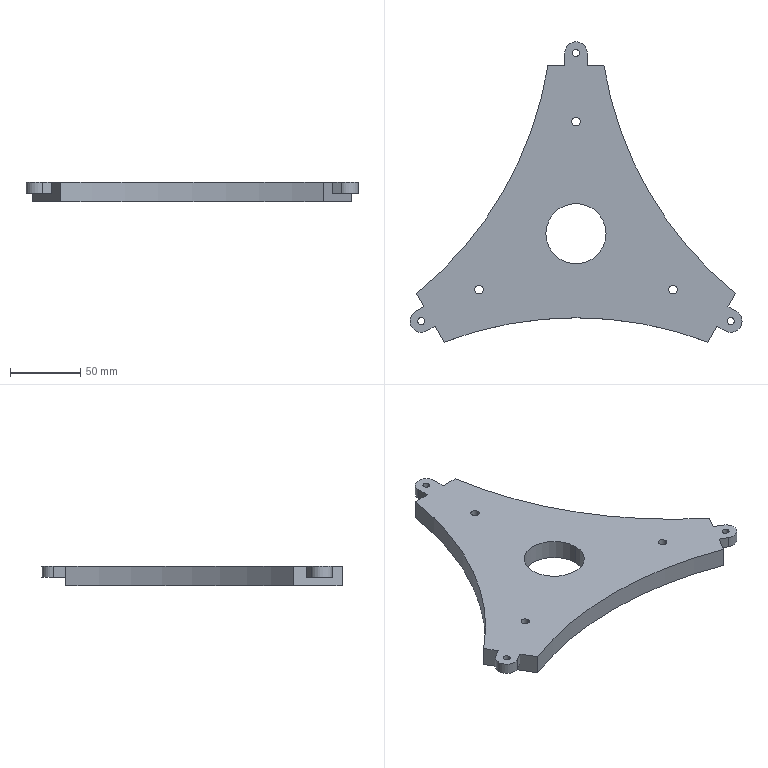Part | SolidWorks | features ICE 3, 3DProfileFeature 2, HoleWzd 2, CirPattern 1, Extrusion 1 | 1 solid | 35 faces | box 237.049 x 214.321 x 14 mm | volume 297445 mm3 | cylinder 21 | plane 14 | commonest cylinder face diameters 5 x6 6 x6 16 x4 526.632 x3 43 x2
STEP:
#1=CARTESIAN_POINT('',(-3.,80.,14.));
#2=VERTEX_POINT('',#1);
#3=CARTESIAN_POINT('',(3.,80.,14.));
#4=VERTEX_POINT('',#3);
#5=CARTESIAN_POINT('',(0.,80.,14.));
#6=DIRECTION('',(0.,0.,1.));
#7=DIRECTION('',(1.,0.,0.));
#8=AXIS2_PLACEMENT_3D('',#5,#6,#7);
#9=CIRCLE('',#8,3.);
#10=EDGE_CURVE('',#2,#4,#9,.T.);
#11=ORIENTED_EDGE('',*,*,#10,.T.);
#12=CARTESIAN_POINT('',(3.,80.,0.));
#13=VERTEX_POINT('',#12);
#14=CARTESIAN_POINT('',(3.,80.,17.));
#15=DIRECTION('',(0.,0.,-1.));
#16=VECTOR('',#15,1000.);
#17=LINE('',#14,#16);
#18=EDGE_CURVE('',#4,#13,#17,.T.);
#19=ORIENTED_EDGE('',*,*,#18,.T.);
#20=CARTESIAN_POINT('',(-3.,80.,0.));
#21=VERTEX_POINT('',#20);
#22=CARTESIAN_POINT('',(0.,80.,0.));
#23=DIRECTION('',(0.,0.,-1.));
#24=DIRECTION('',(-1.,0.,0.));
#25=AXIS2_PLACEMENT_3D('',#22,#23,#24);
#26=CIRCLE('',#25,3.);
#27=EDGE_CURVE('',#13,#21,#26,.T.);
#28=ORIENTED_EDGE('',*,*,#27,.T.);
#29=CARTESIAN_POINT('',(-3.,80.,17.));
#30=DIRECTION('',(0.,0.,-1.));
#31=VECTOR('',#30,1000.);
#32=LINE('',#29,#31);
#33=EDGE_CURVE('',#2,#21,#32,.T.);
#34=ORIENTED_EDGE('',*,*,#33,.F.);
#35=EDGE_LOOP('',(#11,#19,#28,#34));
#36=FACE_OUTER_BOUND('',#35,.T.);
#37=CARTESIAN_POINT('',(0.,80.,17.));
#38=DIRECTION('',(0.,0.,-1.));
#39=DIRECTION('',(-1.,0.,0.));
#40=AXIS2_PLACEMENT_3D('',#37,#38,#39);
#41=CYLINDRICAL_SURFACE('',#40,3.);
#42=ADVANCED_FACE('',(#36),#41,.F.);
#43=CARTESIAN_POINT('',(-72.282,-40.,14.));
#44=VERTEX_POINT('',#43);
#45=CARTESIAN_POINT('',(-66.282,-40.,14.));
#46=VERTEX_POINT('',#45);
#47=CARTESIAN_POINT('',(-69.282,-40.,14.));
#48=DIRECTION('',(0.,0.,1.));
#49=DIRECTION('',(1.,0.,0.));
#50=AXIS2_PLACEMENT_3D('',#47,#48,#49);
#51=CIRCLE('',#50,3.);
#52=EDGE_CURVE('',#44,#46,#51,.T.);
#53=ORIENTED_EDGE('',*,*,#52,.T.);
#54=CARTESIAN_POINT('',(-66.282,-40.,0.));
#55=VERTEX_POINT('',#54);
#56=CARTESIAN_POINT('',(-66.282,-40.,17.));
#57=DIRECTION('',(0.,0.,-1.));
#58=VECTOR('',#57,1000.);
#59=LINE('',#56,#58);
#60=EDGE_CURVE('',#46,#55,#59,.T.);
#61=ORIENTED_EDGE('',*,*,#60,.T.);
#62=CARTESIAN_POINT('',(-72.282,-40.,0.));
#63=VERTEX_POINT('',#62);
#64=CARTESIAN_POINT('',(-69.282,-40.,0.));
#65=DIRECTION('',(0.,0.,-1.));
#66=DIRECTION('',(-1.,0.,0.));
#67=AXIS2_PLACEMENT_3D('',#64,#65,#66);
#68=CIRCLE('',#67,3.);
#69=EDGE_CURVE('',#55,#63,#68,.T.);
#70=ORIENTED_EDGE('',*,*,#69,.T.);
#71=CARTESIAN_POINT('',(-72.282,-40.,17.));
#72=DIRECTION('',(0.,0.,-1.));
#73=VECTOR('',#72,1000.);
#74=LINE('',#71,#73);
#75=EDGE_CURVE('',#44,#63,#74,.T.);
#76=ORIENTED_EDGE('',*,*,#75,.F.);
#77=EDGE_LOOP('',(#53,#61,#70,#76));
#78=FACE_OUTER_BOUND('',#77,.T.);
#79=CARTESIAN_POINT('',(-69.282,-40.,17.));
#80=DIRECTION('',(0.,0.,-1.));
#81=DIRECTION('',(-1.,0.,0.));
#82=AXIS2_PLACEMENT_3D('',#79,#80,#81);
#83=CYLINDRICAL_SURFACE('',#82,3.);
#84=ADVANCED_FACE('',(#78),#83,.F.);
#85=CARTESIAN_POINT('',(66.282,-40.,14.));
#86=VERTEX_POINT('',#85);
#87=CARTESIAN_POINT('',(72.282,-40.,14.));
#88=VERTEX_POINT('',#87);
#89=CARTESIAN_POINT('',(69.282,-40.,14.));
#90=DIRECTION('',(0.,0.,1.));
#91=DIRECTION('',(1.,0.,0.));
#92=AXIS2_PLACEMENT_3D('',#89,#90,#91);
#93=CIRCLE('',#92,3.);
#94=EDGE_CURVE('',#86,#88,#93,.T.);
#95=ORIENTED_EDGE('',*,*,#94,.T.);
#96=CARTESIAN_POINT('',(72.282,-40.,0.));
#97=VERTEX_POINT('',#96);
#98=CARTESIAN_POINT('',(72.282,-40.,17.));
#99=DIRECTION('',(0.,0.,-1.));
#100=VECTOR('',#99,1000.);
#101=LINE('',#98,#100);
#102=EDGE_CURVE('',#88,#97,#101,.T.);
#103=ORIENTED_EDGE('',*,*,#102,.T.);
#104=CARTESIAN_POINT('',(66.282,-40.,0.));
#105=VERTEX_POINT('',#104);
#106=CARTESIAN_POINT('',(69.282,-40.,0.));
#107=DIRECTION('',(0.,0.,-1.));
#108=DIRECTION('',(-1.,0.,0.));
#109=AXIS2_PLACEMENT_3D('',#106,#107,#108);
#110=CIRCLE('',#109,3.);
#111=EDGE_CURVE('',#97,#105,#110,.T.);
#112=ORIENTED_EDGE('',*,*,#111,.T.);
#113=CARTESIAN_POINT('',(66.282,-40.,17.));
#114=DIRECTION('',(0.,0.,-1.));
#115=VECTOR('',#114,1000.);
#116=LINE('',#113,#115);
#117=EDGE_CURVE('',#86,#105,#116,.T.);
#118=ORIENTED_EDGE('',*,*,#117,.F.);
#119=EDGE_LOOP('',(#95,#103,#112,#118));
#120=FACE_OUTER_BOUND('',#119,.T.);
#121=CARTESIAN_POINT('',(69.282,-40.,17.));
#122=DIRECTION('',(0.,0.,-1.));
#123=DIRECTION('',(-1.,0.,0.));
#124=AXIS2_PLACEMENT_3D('',#121,#122,#123);
#125=CYLINDRICAL_SURFACE('',#124,3.);
#126=ADVANCED_FACE('',(#120),#125,.F.);
#127=CARTESIAN_POINT('',(-113.024,-62.434,6.));
#128=VERTEX_POINT('',#127);
#129=CARTESIAN_POINT('',(-108.024,-62.434,6.));
#130=VERTEX_POINT('',#129);
#131=CARTESIAN_POINT('',(-110.524,-62.434,6.));
#132=DIRECTION('',(0.,0.,1.));
#133=DIRECTION('',(1.,0.,0.));
#134=AXIS2_PLACEMENT_3D('',#131,#132,#133);
#135=CIRCLE('',#134,2.5);
#136=EDGE_CURVE('',#128,#130,#135,.T.);
#137=ORIENTED_EDGE('',*,*,#136,.F.);
#138=CARTESIAN_POINT('',(-113.024,-62.434,14.));
#139=VERTEX_POINT('',#138);
#140=CARTESIAN_POINT('',(-113.024,-62.434,14.));
#141=DIRECTION('',(0.,0.,1.));
#142=VECTOR('',#141,1000.);
#143=LINE('',#140,#142);
#144=EDGE_CURVE('',#128,#139,#143,.T.);
#145=ORIENTED_EDGE('',*,*,#144,.T.);
#146=CARTESIAN_POINT('',(-108.024,-62.434,14.));
#147=VERTEX_POINT('',#146);
#148=CARTESIAN_POINT('',(-110.524,-62.434,14.));
#149=DIRECTION('',(0.,0.,1.));
#150=DIRECTION('',(1.,0.,0.));
#151=AXIS2_PLACEMENT_3D('',#148,#149,#150);
#152=CIRCLE('',#151,2.5);
#153=EDGE_CURVE('',#139,#147,#152,.T.);
#154=ORIENTED_EDGE('',*,*,#153,.T.);
#155=CARTESIAN_POINT('',(-108.024,-62.434,14.));
#156=DIRECTION('',(0.,0.,1.));
#157=VECTOR('',#156,1000.);
#158=LINE('',#155,#157);
#159=EDGE_CURVE('',#130,#147,#158,.T.);
#160=ORIENTED_EDGE('',*,*,#159,.F.);
#161=EDGE_LOOP('',(#137,#145,#154,#160));
#162=FACE_OUTER_BOUND('',#161,.T.);
#163=CARTESIAN_POINT('',(-110.524,-62.434,14.));
#164=DIRECTION('',(0.,0.,1.));
#165=DIRECTION('',(1.,0.,0.));
#166=AXIS2_PLACEMENT_3D('',#163,#164,#165);
#167=CYLINDRICAL_SURFACE('',#166,2.5);
#168=ADVANCED_FACE('',(#162),#167,.F.);
#169=CARTESIAN_POINT('',(108.024,-62.434,6.));
#170=VERTEX_POINT('',#169);
#171=CARTESIAN_POINT('',(113.024,-62.434,6.));
#172=VERTEX_POINT('',#171);
#173=CARTESIAN_POINT('',(110.524,-62.434,6.));
#174=DIRECTION('',(0.,0.,1.));
#175=DIRECTION('',(1.,0.,0.));
#176=AXIS2_PLACEMENT_3D('',#173,#174,#175);
#177=CIRCLE('',#176,2.5);
#178=EDGE_CURVE('',#170,#172,#177,.T.);
#179=ORIENTED_EDGE('',*,*,#178,.F.);
#180=CARTESIAN_POINT('',(108.024,-62.434,14.));
#181=VERTEX_POINT('',#180);
#182=CARTESIAN_POINT('',(108.024,-62.434,14.));
#183=DIRECTION('',(0.,0.,1.));
#184=VECTOR('',#183,1000.);
#185=LINE('',#182,#184);
#186=EDGE_CURVE('',#170,#181,#185,.T.);
#187=ORIENTED_EDGE('',*,*,#186,.T.);
#188=CARTESIAN_POINT('',(113.024,-62.434,14.));
#189=VERTEX_POINT('',#188);
#190=CARTESIAN_POINT('',(110.524,-62.434,14.));
#191=DIRECTION('',(0.,0.,1.));
#192=DIRECTION('',(1.,0.,0.));
#193=AXIS2_PLACEMENT_3D('',#190,#191,#192);
#194=CIRCLE('',#193,2.5);
#195=EDGE_CURVE('',#181,#189,#194,.T.);
#196=ORIENTED_EDGE('',*,*,#195,.T.);
#197=CARTESIAN_POINT('',(113.024,-62.434,14.));
#198=DIRECTION('',(0.,0.,1.));
#199=VECTOR('',#198,1000.);
#200=LINE('',#197,#199);
#201=EDGE_CURVE('',#172,#189,#200,.T.);
#202=ORIENTED_EDGE('',*,*,#201,.F.);
#203=EDGE_LOOP('',(#179,#187,#196,#202));
#204=FACE_OUTER_BOUND('',#203,.T.);
#205=CARTESIAN_POINT('',(110.524,-62.434,14.));
#206=DIRECTION('',(0.,0.,1.));
#207=DIRECTION('',(1.,0.,0.));
#208=AXIS2_PLACEMENT_3D('',#205,#206,#207);
#209=CYLINDRICAL_SURFACE('',#208,2.5);
#210=ADVANCED_FACE('',(#204),#209,.F.);
#211=CARTESIAN_POINT('',(21.5,0.,14.));
#212=VERTEX_POINT('',#211);
#213=CARTESIAN_POINT('',(-21.5,0.,14.));
#214=VERTEX_POINT('',#213);
#215=CARTESIAN_POINT('',(0.,0.,14.));
#216=DIRECTION('',(0.,0.,-1.));
#217=DIRECTION('',(-1.,0.,0.));
#218=AXIS2_PLACEMENT_3D('',#215,#216,#217);
#219=CIRCLE('',#218,21.5);
#220=EDGE_CURVE('',#212,#214,#219,.T.);
#221=ORIENTED_EDGE('',*,*,#220,.F.);
#222=CARTESIAN_POINT('',(21.5,0.,0.));
#223=VERTEX_POINT('',#222);
#224=CARTESIAN_POINT('',(21.5,0.,14.));
#225=DIRECTION('',(0.,0.,-1.));
#226=VECTOR('',#225,1000.);
#227=LINE('',#224,#226);
#228=EDGE_CURVE('',#212,#223,#227,.T.);
#229=ORIENTED_EDGE('',*,*,#228,.T.);
#230=CARTESIAN_POINT('',(-21.5,0.,0.));
#231=VERTEX_POINT('',#230);
#232=CARTESIAN_POINT('',(0.,0.,0.));
#233=DIRECTION('',(0.,0.,-1.));
#234=DIRECTION('',(-1.,0.,0.));
#235=AXIS2_PLACEMENT_3D('',#232,#233,#234);
#236=CIRCLE('',#235,21.5);
#237=EDGE_CURVE('',#223,#231,#236,.T.);
#238=ORIENTED_EDGE('',*,*,#237,.T.);
#239=CARTESIAN_POINT('',(-21.5,0.,14.));
#240=DIRECTION('',(0.,0.,-1.));
#241=VECTOR('',#240,1000.);
#242=LINE('',#239,#241);
#243=EDGE_CURVE('',#214,#231,#242,.T.);
#244=ORIENTED_EDGE('',*,*,#243,.F.);
#245=EDGE_LOOP('',(#221,#229,#238,#244));
#246=FACE_OUTER_BOUND('',#245,.T.);
#247=CARTESIAN_POINT('',(0.,0.,14.));
#248=DIRECTION('',(0.,0.,-1.));
#249=DIRECTION('',(-1.,0.,0.));
#250=AXIS2_PLACEMENT_3D('',#247,#248,#249);
#251=CYLINDRICAL_SURFACE('',#250,21.5);
#252=ADVANCED_FACE('',(#246),#251,.F.);
#253=CARTESIAN_POINT('',(-2.5,129.,14.));
#254=VERTEX_POINT('',#253);
#255=CARTESIAN_POINT('',(2.5,129.,14.));
#256=VERTEX_POINT('',#255);
#257=CARTESIAN_POINT('',(0.,129.,14.));
#258=DIRECTION('',(0.,0.,1.));
#259=DIRECTION('',(1.,0.,0.));
#260=AXIS2_PLACEMENT_3D('',#257,#258,#259);
#261=CIRCLE('',#260,2.5);
#262=EDGE_CURVE('',#254,#256,#261,.T.);
#263=ORIENTED_EDGE('',*,*,#262,.T.);
#264=CARTESIAN_POINT('',(2.5,129.,6.));
#265=VERTEX_POINT('',#264);
#266=CARTESIAN_POINT('',(2.5,129.,6.));
#267=DIRECTION('',(0.,0.,-1.));
#268=VECTOR('',#267,1000.);
#269=LINE('',#266,#268);
#270=EDGE_CURVE('',#256,#265,#269,.T.);
#271=ORIENTED_EDGE('',*,*,#270,.T.);
#272=CARTESIAN_POINT('',(-2.5,129.,6.));
#273=VERTEX_POINT('',#272);
#274=CARTESIAN_POINT('',(0.,129.,6.));
#275=DIRECTION('',(0.,0.,-1.));
#276=DIRECTION('',(-1.,0.,0.));
#277=AXIS2_PLACEMENT_3D('',#274,#275,#276);
#278=CIRCLE('',#277,2.5);
#279=EDGE_CURVE('',#265,#273,#278,.T.);
#280=ORIENTED_EDGE('',*,*,#279,.T.);
#281=CARTESIAN_POINT('',(-2.5,129.,6.));
#282=DIRECTION('',(0.,0.,-1.));
#283=VECTOR('',#282,1000.);
#284=LINE('',#281,#283);
#285=EDGE_CURVE('',#254,#273,#284,.T.);
#286=ORIENTED_EDGE('',*,*,#285,.F.);
#287=EDGE_LOOP('',(#263,#271,#280,#286));
#288=FACE_OUTER_BOUND('',#287,.T.);
#289=CARTESIAN_POINT('',(0.,129.,6.));
#290=DIRECTION('',(0.,0.,-1.));
#291=DIRECTION('',(-1.,0.,0.));
#292=AXIS2_PLACEMENT_3D('',#289,#290,#291);
#293=CYLINDRICAL_SURFACE('',#292,2.5);
#294=ADVANCED_FACE('',(#288),#293,.F.);
#295=CARTESIAN_POINT('',(106.524,-69.362,6.));
#296=VERTEX_POINT('',#295);
#297=CARTESIAN_POINT('',(118.524,-62.434,6.));
#298=VERTEX_POINT('',#297);
#299=CARTESIAN_POINT('',(110.524,-62.434,6.));
#300=DIRECTION('',(0.,0.,1.));
#301=DIRECTION('',(-0.5,-0.866,0.));
#302=AXIS2_PLACEMENT_3D('',#299,#300,#301);
#303=CIRCLE('',#302,8.);
#304=EDGE_CURVE('',#296,#298,#303,.T.);
#305=ORIENTED_EDGE('',*,*,#304,.T.);
#306=CARTESIAN_POINT('',(118.524,-62.434,14.));
#307=VERTEX_POINT('',#306);
#308=CARTESIAN_POINT('',(118.524,-62.434,6.));
#309=DIRECTION('',(0.,0.,1.));
#310=VECTOR('',#309,1000.);
#311=LINE('',#308,#310);
#312=EDGE_CURVE('',#298,#307,#311,.T.);
#313=ORIENTED_EDGE('',*,*,#312,.T.);
#314=CARTESIAN_POINT('',(106.524,-69.362,14.));
#315=VERTEX_POINT('',#314);
#316=CARTESIAN_POINT('',(110.524,-62.434,14.));
#317=DIRECTION('',(0.,0.,1.));
#318=DIRECTION('',(-0.5,-0.866,0.));
#319=AXIS2_PLACEMENT_3D('',#316,#317,#318);
#320=CIRCLE('',#319,8.);
#321=EDGE_CURVE('',#315,#307,#320,.T.);
#322=ORIENTED_EDGE('',*,*,#321,.F.);
#323=CARTESIAN_POINT('',(106.524,-69.362,6.));
#324=DIRECTION('',(0.,0.,1.));
#325=VECTOR('',#324,1000.);
#326=LINE('',#323,#325);
#327=EDGE_CURVE('',#296,#315,#326,.T.);
#328=ORIENTED_EDGE('',*,*,#327,.F.);
#329=EDGE_LOOP('',(#305,#313,#322,#328));
#330=FACE_OUTER_BOUND('',#329,.T.);
#331=CARTESIAN_POINT('',(110.524,-62.434,6.));
#332=DIRECTION('',(0.,0.,1.));
#333=DIRECTION('',(1.,0.,0.));
#334=AXIS2_PLACEMENT_3D('',#331,#332,#333);
#335=CYLINDRICAL_SURFACE('',#334,8.);
#336=ADVANCED_FACE('',(#330),#335,.T.);
#337=CARTESIAN_POINT('',(-8.,120.,6.));
#338=VERTEX_POINT('',#337);
#339=CARTESIAN_POINT('',(-8.,120.,14.));
#340=VERTEX_POINT('',#339);
#341=CARTESIAN_POINT('',(-8.,120.,6.));
#342=DIRECTION('',(0.,0.,1.));
#343=VECTOR('',#342,1000.);
#344=LINE('',#341,#343);
#345=EDGE_CURVE('',#338,#340,#344,.T.);
#346=ORIENTED_EDGE('',*,*,#345,.F.);
#347=CARTESIAN_POINT('',(8.,120.,6.));
#348=VERTEX_POINT('',#347);
#349=CARTESIAN_POINT('',(0.,120.,6.));
#350=DIRECTION('',(-1.,0.,0.));
#351=VECTOR('',#350,1000.);
#352=LINE('',#349,#351);
#353=EDGE_CURVE('',#348,#338,#352,.T.);
#354=ORIENTED_EDGE('',*,*,#353,.F.);
#355=CARTESIAN_POINT('',(8.,120.,14.));
#356=VERTEX_POINT('',#355);
#357=CARTESIAN_POINT('',(8.,120.,6.));
#358=DIRECTION('',(0.,0.,1.));
#359=VECTOR('',#358,1000.);
#360=LINE('',#357,#359);
#361=EDGE_CURVE('',#348,#356,#360,.T.);
#362=ORIENTED_EDGE('',*,*,#361,.T.);
#363=CARTESIAN_POINT('',(20.,120.,14.));
#364=VERTEX_POINT('',#363);
#365=CARTESIAN_POINT('',(-20.,120.,14.));
#366=DIRECTION('',(-1.,0.,0.));
#367=VECTOR('',#366,1000.);
#368=LINE('',#365,#367);
#369=EDGE_CURVE('',#364,#356,#368,.T.);
#370=ORIENTED_EDGE('',*,*,#369,.F.);
#371=CARTESIAN_POINT('',(20.,120.,0.));
#372=VERTEX_POINT('',#371);
#373=CARTESIAN_POINT('',(20.,120.,14.));
#374=DIRECTION('',(0.,0.,-1.));
#375=VECTOR('',#374,1000.);
#376=LINE('',#373,#375);
#377=EDGE_CURVE('',#364,#372,#376,.T.);
#378=ORIENTED_EDGE('',*,*,#377,.T.);
#379=CARTESIAN_POINT('',(-20.,120.,0.));
#380=VERTEX_POINT('',#379);
#381=CARTESIAN_POINT('',(-20.,120.,0.));
#382=DIRECTION('',(-1.,0.,0.));
#383=VECTOR('',#382,1000.);
#384=LINE('',#381,#383);
#385=EDGE_CURVE('',#372,#380,#384,.T.);
#386=ORIENTED_EDGE('',*,*,#385,.T.);
#387=CARTESIAN_POINT('',(-20.,120.,14.));
#388=VERTEX_POINT('',#387);
#389=CARTESIAN_POINT('',(-20.,120.,14.));
#390=DIRECTION('',(0.,0.,-1.));
#391=VECTOR('',#390,1000.);
#392=LINE('',#389,#391);
#393=EDGE_CURVE('',#388,#380,#392,.T.);
#394=ORIENTED_EDGE('',*,*,#393,.F.);
#395=CARTESIAN_POINT('',(-20.,120.,14.));
#396=DIRECTION('',(-1.,0.,0.));
#397=VECTOR('',#396,1000.);
#398=LINE('',#395,#397);
#399=EDGE_CURVE('',#340,#388,#398,.T.);
#400=ORIENTED_EDGE('',*,*,#399,.F.);
#401=EDGE_LOOP('',(#346,#354,#362,#370,#378,#386,#394,#400));
#402=FACE_OUTER_BOUND('',#401,.T.);
#403=CARTESIAN_POINT('',(-20.,120.,14.));
#404=DIRECTION('',(0.,-1.,0.));
#405=DIRECTION('',(0.,0.,-1.));
#406=AXIS2_PLACEMENT_3D('',#403,#404,#405);
#407=PLANE('',#406);
#408=ADVANCED_FACE('',(#402),#407,.F.);
#409=CARTESIAN_POINT('',(113.923,-42.679,0.));
#410=VERTEX_POINT('',#409);
#411=CARTESIAN_POINT('',(280.,161.658,0.));
#412=DIRECTION('',(0.,0.,-1.));
#413=DIRECTION('',(1.,0.,0.));
#414=AXIS2_PLACEMENT_3D('',#411,#412,#413);
#415=CIRCLE('',#414,263.316);
#416=EDGE_CURVE('',#410,#372,#415,.T.);
#417=ORIENTED_EDGE('',*,*,#416,.T.);
#418=ORIENTED_EDGE('',*,*,#377,.F.);
#419=CARTESIAN_POINT('',(113.923,-42.679,14.));
#420=VERTEX_POINT('',#419);
#421=CARTESIAN_POINT('',(280.,161.658,14.));
#422=DIRECTION('',(0.,0.,-1.));
#423=DIRECTION('',(1.,0.,0.));
#424=AXIS2_PLACEMENT_3D('',#421,#422,#423);
#425=CIRCLE('',#424,263.316);
#426=EDGE_CURVE('',#420,#364,#425,.T.);
#427=ORIENTED_EDGE('',*,*,#426,.F.);
#428=CARTESIAN_POINT('',(113.923,-42.679,14.));
#429=DIRECTION('',(0.,0.,-1.));
#430=VECTOR('',#429,1000.);
#431=LINE('',#428,#430);
#432=EDGE_CURVE('',#420,#410,#431,.T.);
#433=ORIENTED_EDGE('',*,*,#432,.T.);
#434=EDGE_LOOP('',(#417,#418,#427,#433));
#435=FACE_OUTER_BOUND('',#434,.T.);
#436=CARTESIAN_POINT('',(280.,161.658,14.));
#437=DIRECTION('',(0.,0.,-1.));
#438=DIRECTION('',(-1.,0.,0.));
#439=AXIS2_PLACEMENT_3D('',#436,#437,#438);
#440=CYLINDRICAL_SURFACE('',#439,263.316);
#441=ADVANCED_FACE('',(#435),#440,.F.);
#442=CARTESIAN_POINT('',(-113.923,-42.679,0.));
#443=VERTEX_POINT('',#442);
#444=CARTESIAN_POINT('',(-280.,161.658,0.));
#445=DIRECTION('',(0.,0.,-1.));
#446=DIRECTION('',(1.,0.,0.));
#447=AXIS2_PLACEMENT_3D('',#444,#445,#446);
#448=CIRCLE('',#447,263.316);
#449=EDGE_CURVE('',#380,#443,#448,.T.);
#450=ORIENTED_EDGE('',*,*,#449,.T.);
#451=CARTESIAN_POINT('',(-113.923,-42.679,14.));
#452=VERTEX_POINT('',#451);
#453=CARTESIAN_POINT('',(-113.923,-42.679,14.));
#454=DIRECTION('',(0.,0.,-1.));
#455=VECTOR('',#454,1000.);
#456=LINE('',#453,#455);
#457=EDGE_CURVE('',#452,#443,#456,.T.);
#458=ORIENTED_EDGE('',*,*,#457,.F.);
#459=CARTESIAN_POINT('',(-280.,161.658,14.));
#460=DIRECTION('',(0.,0.,-1.));
#461=DIRECTION('',(1.,0.,0.));
#462=AXIS2_PLACEMENT_3D('',#459,#460,#461);
#463=CIRCLE('',#462,263.316);
#464=EDGE_CURVE('',#388,#452,#463,.T.);
#465=ORIENTED_EDGE('',*,*,#464,.F.);
#466=ORIENTED_EDGE('',*,*,#393,.T.);
#467=EDGE_LOOP('',(#450,#458,#465,#466));
#468=FACE_OUTER_BOUND('',#467,.T.);
#469=CARTESIAN_POINT('',(-280.,161.658,14.));
#470=DIRECTION('',(0.,0.,-1.));
#471=DIRECTION('',(-1.,0.,0.));
#472=AXIS2_PLACEMENT_3D('',#469,#470,#471);
#473=CYLINDRICAL_SURFACE('',#472,263.316);
#474=ADVANCED_FACE('',(#468),#473,.F.);
#475=CARTESIAN_POINT('',(-108.519,-52.039,6.));
#476=VERTEX_POINT('',#475);
#477=CARTESIAN_POINT('',(-100.519,-65.895,6.));
#478=VERTEX_POINT('',#477);
#479=CARTESIAN_POINT('',(-93.923,-77.321,6.));
#480=DIRECTION('',(0.5,-0.866,0.));
#481=VECTOR('',#480,1000.);
#482=LINE('',#479,#481);
#483=EDGE_CURVE('',#476,#478,#482,.T.);
#484=ORIENTED_EDGE('',*,*,#483,.F.);
#485=CARTESIAN_POINT('',(-108.519,-52.039,14.));
#486=VERTEX_POINT('',#485);
#487=CARTESIAN_POINT('',(-108.519,-52.039,14.));
#488=DIRECTION('',(0.,0.,1.));
#489=VECTOR('',#488,1000.);
#490=LINE('',#487,#489);
#491=EDGE_CURVE('',#476,#486,#490,.T.);
#492=ORIENTED_EDGE('',*,*,#491,.T.);
#493=CARTESIAN_POINT('',(-93.923,-77.321,14.));
#494=DIRECTION('',(0.5,-0.866,0.));
#495=VECTOR('',#494,1000.);
#496=LINE('',#493,#495);
#497=EDGE_CURVE('',#452,#486,#496,.T.);
#498=ORIENTED_EDGE('',*,*,#497,.F.);
#499=ORIENTED_EDGE('',*,*,#457,.T.);
#500=CARTESIAN_POINT('',(-93.923,-77.321,0.));
#501=VERTEX_POINT('',#500);
#502=CARTESIAN_POINT('',(-93.923,-77.321,0.));
#503=DIRECTION('',(0.5,-0.866,0.));
#504=VECTOR('',#503,1000.);
#505=LINE('',#502,#504);
#506=EDGE_CURVE('',#443,#501,#505,.T.);
#507=ORIENTED_EDGE('',*,*,#506,.T.);
#508=CARTESIAN_POINT('',(-93.923,-77.321,14.));
#509=VERTEX_POINT('',#508);
#510=CARTESIAN_POINT('',(-93.923,-77.321,14.));
#511=DIRECTION('',(0.,0.,-1.));
#512=VECTOR('',#511,1000.);
#513=LINE('',#510,#512);
#514=EDGE_CURVE('',#509,#501,#513,.T.);
#515=ORIENTED_EDGE('',*,*,#514,.F.);
#516=CARTESIAN_POINT('',(-100.519,-65.895,14.));
#517=VERTEX_POINT('',#516);
#518=CARTESIAN_POINT('',(-93.923,-77.321,14.));
#519=DIRECTION('',(0.5,-0.866,0.));
#520=VECTOR('',#519,1000.);
#521=LINE('',#518,#520);
#522=EDGE_CURVE('',#517,#509,#521,.T.);
#523=ORIENTED_EDGE('',*,*,#522,.F.);
#524=CARTESIAN_POINT('',(-100.519,-65.895,14.));
#525=DIRECTION('',(0.,0.,1.));
#526=VECTOR('',#525,1000.);
#527=LINE('',#524,#526);
#528=EDGE_CURVE('',#478,#517,#527,.T.);
#529=ORIENTED_EDGE('',*,*,#528,.F.);
#530=EDGE_LOOP('',(#484,#492,#498,#499,#507,#515,#523,#529));
#531=FACE_OUTER_BOUND('',#530,.T.);
#532=CARTESIAN_POINT('',(-93.923,-77.321,14.));
#533=DIRECTION('',(0.866,0.5,0.));
#534=DIRECTION('',(-0.5,0.866,0.));
#535=AXIS2_PLACEMENT_3D('',#532,#533,#534);
#536=PLANE('',#535);
#537=ADVANCED_FACE('',(#531),#536,.F.);
#538=CARTESIAN_POINT('',(93.923,-77.321,0.));
#539=VERTEX_POINT('',#538);
#540=CARTESIAN_POINT('',(0.,-323.316,0.));
#541=DIRECTION('',(0.,0.,-1.));
#542=DIRECTION('',(1.,0.,0.));
#543=AXIS2_PLACEMENT_3D('',#540,#541,#542);
#544=CIRCLE('',#543,263.316);
#545=EDGE_CURVE('',#501,#539,#544,.T.);
#546=ORIENTED_EDGE('',*,*,#545,.T.);
#547=CARTESIAN_POINT('',(93.923,-77.321,14.));
#548=VERTEX_POINT('',#547);
#549=CARTESIAN_POINT('',(93.923,-77.321,14.));
#550=DIRECTION('',(0.,0.,-1.));
#551=VECTOR('',#550,1000.);
#552=LINE('',#549,#551);
#553=EDGE_CURVE('',#548,#539,#552,.T.);
#554=ORIENTED_EDGE('',*,*,#553,.F.);
#555=CARTESIAN_POINT('',(0.,-323.316,14.));
#556=DIRECTION('',(0.,0.,-1.));
#557=DIRECTION('',(1.,0.,0.));
#558=AXIS2_PLACEMENT_3D('',#555,#556,#557);
#559=CIRCLE('',#558,263.316);
#560=EDGE_CURVE('',#509,#548,#559,.T.);
#561=ORIENTED_EDGE('',*,*,#560,.F.);
#562=ORIENTED_EDGE('',*,*,#514,.T.);
#563=EDGE_LOOP('',(#546,#554,#561,#562));
#564=FACE_OUTER_BOUND('',#563,.T.);
#565=CARTESIAN_POINT('',(0.,-323.316,14.));
#566=DIRECTION('',(0.,0.,-1.));
#567=DIRECTION('',(-1.,0.,0.));
#568=AXIS2_PLACEMENT_3D('',#565,#566,#567);
#569=CYLINDRICAL_SURFACE('',#568,263.316);
#570=ADVANCED_FACE('',(#564),#569,.F.);
#571=CARTESIAN_POINT('',(100.519,-65.895,6.));
#572=VERTEX_POINT('',#571);
#573=CARTESIAN_POINT('',(108.519,-52.039,6.));
#574=VERTEX_POINT('',#573);
#575=CARTESIAN_POINT('',(113.923,-42.679,6.));
#576=DIRECTION('',(0.5,0.866,0.));
#577=VECTOR('',#576,1000.);
#578=LINE('',#575,#577);
#579=EDGE_CURVE('',#572,#574,#578,.T.);
#580=ORIENTED_EDGE('',*,*,#579,.F.);
#581=CARTESIAN_POINT('',(100.519,-65.895,14.));
#582=VERTEX_POINT('',#581);
#583=CARTESIAN_POINT('',(100.519,-65.895,14.));
#584=DIRECTION('',(0.,0.,1.));
#585=VECTOR('',#584,1000.);
#586=LINE('',#583,#585);
#587=EDGE_CURVE('',#572,#582,#586,.T.);
#588=ORIENTED_EDGE('',*,*,#587,.T.);
#589=CARTESIAN_POINT('',(113.923,-42.679,14.));
#590=DIRECTION('',(0.5,0.866,0.));
#591=VECTOR('',#590,1000.);
#592=LINE('',#589,#591);
#593=EDGE_CURVE('',#548,#582,#592,.T.);
#594=ORIENTED_EDGE('',*,*,#593,.F.);
#595=ORIENTED_EDGE('',*,*,#553,.T.);
#596=CARTESIAN_POINT('',(113.923,-42.679,0.));
#597=DIRECTION('',(0.5,0.866,0.));
#598=VECTOR('',#597,1000.);
#599=LINE('',#596,#598);
#600=EDGE_CURVE('',#539,#410,#599,.T.);
#601=ORIENTED_EDGE('',*,*,#600,.T.);
#602=ORIENTED_EDGE('',*,*,#432,.F.);
#603=CARTESIAN_POINT('',(108.519,-52.039,14.));
#604=VERTEX_POINT('',#603);
#605=CARTESIAN_POINT('',(113.923,-42.679,14.));
#606=DIRECTION('',(0.5,0.866,0.));
#607=VECTOR('',#606,1000.);
#608=LINE('',#605,#607);
#609=EDGE_CURVE('',#604,#420,#608,.T.);
#610=ORIENTED_EDGE('',*,*,#609,.F.);
#611=CARTESIAN_POINT('',(108.519,-52.039,14.));
#612=DIRECTION('',(0.,0.,1.));
#613=VECTOR('',#612,1000.);
#614=LINE('',#611,#613);
#615=EDGE_CURVE('',#574,#604,#614,.T.);
#616=ORIENTED_EDGE('',*,*,#615,.F.);
#617=EDGE_LOOP('',(#580,#588,#594,#595,#601,#602,#610,#616));
#618=FACE_OUTER_BOUND('',#617,.T.);
#619=CARTESIAN_POINT('',(113.923,-42.679,14.));
#620=DIRECTION('',(-0.866,0.5,0.));
#621=DIRECTION('',(-0.5,-0.866,0.));
#622=AXIS2_PLACEMENT_3D('',#619,#620,#621);
#623=PLANE('',#622);
#624=ADVANCED_FACE('',(#618),#623,.F.);
#625=ORIENTED_EDGE('',*,*,#10,.F.);
#626=CARTESIAN_POINT('',(0.,80.,14.));
#627=DIRECTION('',(0.,0.,1.));
#628=DIRECTION('',(1.,0.,0.));
#629=AXIS2_PLACEMENT_3D('',#626,#627,#628);
#630=CIRCLE('',#629,3.);
#631=EDGE_CURVE('',#4,#2,#630,.T.);
#632=ORIENTED_EDGE('',*,*,#631,.F.);
#633=EDGE_LOOP('',(#625,#632));
#634=FACE_BOUND('',#633,.T.);
#635=ORIENTED_EDGE('',*,*,#52,.F.);
#636=CARTESIAN_POINT('',(-69.282,-40.,14.));
#637=DIRECTION('',(0.,0.,1.));
#638=DIRECTION('',(1.,0.,0.));
#639=AXIS2_PLACEMENT_3D('',#636,#637,#638);
#640=CIRCLE('',#639,3.);
#641=EDGE_CURVE('',#46,#44,#640,.T.);
#642=ORIENTED_EDGE('',*,*,#641,.F.);
#643=EDGE_LOOP('',(#635,#642));
#644=FACE_BOUND('',#643,.T.);
#645=ORIENTED_EDGE('',*,*,#94,.F.);
#646=CARTESIAN_POINT('',(69.282,-40.,14.));
#647=DIRECTION('',(0.,0.,1.));
#648=DIRECTION('',(1.,0.,0.));
#649=AXIS2_PLACEMENT_3D('',#646,#647,#648);
#650=CIRCLE('',#649,3.);
#651=EDGE_CURVE('',#88,#86,#650,.T.);
#652=ORIENTED_EDGE('',*,*,#651,.F.);
#653=EDGE_LOOP('',(#645,#652));
#654=FACE_BOUND('',#653,.T.);
#655=CARTESIAN_POINT('',(-110.524,-62.434,14.));
#656=DIRECTION('',(0.,0.,1.));
#657=DIRECTION('',(1.,0.,0.));
#658=AXIS2_PLACEMENT_3D('',#655,#656,#657);
#659=CIRCLE('',#658,2.5);
#660=EDGE_CURVE('',#147,#139,#659,.T.);
#661=ORIENTED_EDGE('',*,*,#660,.F.);
#662=ORIENTED_EDGE('',*,*,#153,.F.);
#663=EDGE_LOOP('',(#661,#662));
#664=FACE_BOUND('',#663,.T.);
#665=CARTESIAN_POINT('',(110.524,-62.434,14.));
#666=DIRECTION('',(0.,0.,1.));
#667=DIRECTION('',(1.,0.,0.));
#668=AXIS2_PLACEMENT_3D('',#665,#666,#667);
#669=CIRCLE('',#668,2.5);
#670=EDGE_CURVE('',#189,#181,#669,.T.);
#671=ORIENTED_EDGE('',*,*,#670,.F.);
#672=ORIENTED_EDGE('',*,*,#195,.F.);
#673=EDGE_LOOP('',(#671,#672));
#674=FACE_BOUND('',#673,.T.);
#675=CARTESIAN_POINT('',(0.,0.,14.));
#676=DIRECTION('',(0.,0.,-1.));
#677=DIRECTION('',(-1.,0.,0.));
#678=AXIS2_PLACEMENT_3D('',#675,#676,#677);
#679=CIRCLE('',#678,21.5);
#680=EDGE_CURVE('',#214,#212,#679,.T.);
#681=ORIENTED_EDGE('',*,*,#680,.T.);
#682=ORIENTED_EDGE('',*,*,#220,.T.);
#683=EDGE_LOOP('',(#681,#682));
#684=FACE_BOUND('',#683,.T.);
#685=ORIENTED_EDGE('',*,*,#262,.F.);
#686=CARTESIAN_POINT('',(0.,129.,14.));
#687=DIRECTION('',(0.,0.,1.));
#688=DIRECTION('',(1.,0.,0.));
#689=AXIS2_PLACEMENT_3D('',#686,#687,#688);
#690=CIRCLE('',#689,2.5);
#691=EDGE_CURVE('',#256,#254,#690,.T.);
#692=ORIENTED_EDGE('',*,*,#691,.F.);
#693=EDGE_LOOP('',(#685,#692));
#694=FACE_BOUND('',#693,.T.);
#695=ORIENTED_EDGE('',*,*,#593,.T.);
#696=CARTESIAN_POINT('',(-5.193,-4.862,14.));
#697=DIRECTION('',(0.866,-0.5,0.));
#698=VECTOR('',#697,1000.);
#699=LINE('',#696,#698);
#700=EDGE_CURVE('',#582,#315,#699,.T.);
#701=ORIENTED_EDGE('',*,*,#700,.T.);
#702=ORIENTED_EDGE('',*,*,#321,.T.);
#703=CARTESIAN_POINT('',(114.524,-55.506,14.));
#704=VERTEX_POINT('',#703);
#705=CARTESIAN_POINT('',(110.524,-62.434,14.));
#706=DIRECTION('',(0.,0.,1.));
#707=DIRECTION('',(-0.5,-0.866,0.));
#708=AXIS2_PLACEMENT_3D('',#705,#706,#707);
#709=CIRCLE('',#708,8.);
#710=EDGE_CURVE('',#307,#704,#709,.T.);
#711=ORIENTED_EDGE('',*,*,#710,.T.);
#712=CARTESIAN_POINT('',(2.807,8.994,14.));
#713=DIRECTION('',(0.866,-0.5,0.));
#714=VECTOR('',#713,1000.);
#715=LINE('',#712,#714);
#716=EDGE_CURVE('',#604,#704,#715,.T.);
#717=ORIENTED_EDGE('',*,*,#716,.F.);
#718=ORIENTED_EDGE('',*,*,#609,.T.);
#719=ORIENTED_EDGE('',*,*,#426,.T.);
#720=ORIENTED_EDGE('',*,*,#369,.T.);
#721=CARTESIAN_POINT('',(8.,129.,14.));
#722=VERTEX_POINT('',#721);
#723=CARTESIAN_POINT('',(8.,0.,14.));
#724=DIRECTION('',(0.,1.,0.));
#725=VECTOR('',#724,1000.);
#726=LINE('',#723,#725);
#727=EDGE_CURVE('',#356,#722,#726,.T.);
#728=ORIENTED_EDGE('',*,*,#727,.T.);
#729=CARTESIAN_POINT('',(-8.,129.,14.));
#730=VERTEX_POINT('',#729);
#731=CARTESIAN_POINT('',(0.,129.,14.));
#732=DIRECTION('',(0.,0.,1.));
#733=DIRECTION('',(1.,0.,0.));
#734=AXIS2_PLACEMENT_3D('',#731,#732,#733);
#735=CIRCLE('',#734,8.);
#736=EDGE_CURVE('',#722,#730,#735,.T.);
#737=ORIENTED_EDGE('',*,*,#736,.T.);
#738=CARTESIAN_POINT('',(-8.,0.,14.));
#739=DIRECTION('',(0.,1.,0.));
#740=VECTOR('',#739,1000.);
#741=LINE('',#738,#740);
#742=EDGE_CURVE('',#340,#730,#741,.T.);
#743=ORIENTED_EDGE('',*,*,#742,.F.);
#744=ORIENTED_EDGE('',*,*,#399,.T.);
#745=ORIENTED_EDGE('',*,*,#464,.T.);
#746=ORIENTED_EDGE('',*,*,#497,.T.);
#747=CARTESIAN_POINT('',(-114.524,-55.506,14.));
#748=VERTEX_POINT('',#747);
#749=CARTESIAN_POINT('',(-2.807,8.994,14.));
#750=DIRECTION('',(-0.866,-0.5,0.));
#751=VECTOR('',#750,1000.);
#752=LINE('',#749,#751);
#753=EDGE_CURVE('',#486,#748,#752,.T.);
#754=ORIENTED_EDGE('',*,*,#753,.T.);
#755=CARTESIAN_POINT('',(-106.524,-69.362,14.));
#756=VERTEX_POINT('',#755);
#757=CARTESIAN_POINT('',(-110.524,-62.434,14.));
#758=DIRECTION('',(0.,0.,1.));
#759=DIRECTION('',(-0.5,0.866,0.));
#760=AXIS2_PLACEMENT_3D('',#757,#758,#759);
#761=CIRCLE('',#760,8.);
#762=EDGE_CURVE('',#748,#756,#761,.T.);
#763=ORIENTED_EDGE('',*,*,#762,.T.);
#764=CARTESIAN_POINT('',(5.193,-4.862,14.));
#765=DIRECTION('',(-0.866,-0.5,0.));
#766=VECTOR('',#765,1000.);
#767=LINE('',#764,#766);
#768=EDGE_CURVE('',#517,#756,#767,.T.);
#769=ORIENTED_EDGE('',*,*,#768,.F.);
#770=ORIENTED_EDGE('',*,*,#522,.T.);
#771=ORIENTED_EDGE('',*,*,#560,.T.);
#772=EDGE_LOOP('',(#695,#701,#702,#711,#717,#718,#719,#720,#728,#737,#743,#744,#745,#746,#754,#763,#769,#770,#771));
#773=FACE_OUTER_BOUND('',#772,.T.);
#774=CARTESIAN_POINT('',(280.,161.658,14.));
#775=DIRECTION('',(0.,0.,1.));
#776=DIRECTION('',(1.,0.,0.));
#777=AXIS2_PLACEMENT_3D('',#774,#775,#776);
#778=PLANE('',#777);
#779=ADVANCED_FACE('',(#634,#644,#654,#664,#674,#684,#694,#773),#778,.T.);
#780=CARTESIAN_POINT('',(0.,80.,0.));
#781=DIRECTION('',(0.,0.,-1.));
#782=DIRECTION('',(-1.,0.,0.));
#783=AXIS2_PLACEMENT_3D('',#780,#781,#782);
#784=CIRCLE('',#783,3.);
#785=EDGE_CURVE('',#21,#13,#784,.T.);
#786=ORIENTED_EDGE('',*,*,#785,.F.);
#787=ORIENTED_EDGE('',*,*,#27,.F.);
#788=EDGE_LOOP('',(#786,#787));
#789=FACE_BOUND('',#788,.T.);
#790=CARTESIAN_POINT('',(-69.282,-40.,0.));
#791=DIRECTION('',(0.,0.,-1.));
#792=DIRECTION('',(-1.,0.,0.));
#793=AXIS2_PLACEMENT_3D('',#790,#791,#792);
#794=CIRCLE('',#793,3.);
#795=EDGE_CURVE('',#63,#55,#794,.T.);
#796=ORIENTED_EDGE('',*,*,#795,.F.);
#797=ORIENTED_EDGE('',*,*,#69,.F.);
#798=EDGE_LOOP('',(#796,#797));
#799=FACE_BOUND('',#798,.T.);
#800=CARTESIAN_POINT('',(69.282,-40.,0.));
#801=DIRECTION('',(0.,0.,-1.));
#802=DIRECTION('',(-1.,0.,0.));
#803=AXIS2_PLACEMENT_3D('',#800,#801,#802);
#804=CIRCLE('',#803,3.);
#805=EDGE_CURVE('',#105,#97,#804,.T.);
#806=ORIENTED_EDGE('',*,*,#805,.F.);
#807=ORIENTED_EDGE('',*,*,#111,.F.);
#808=EDGE_LOOP('',(#806,#807));
#809=FACE_BOUND('',#808,.T.);
#810=CARTESIAN_POINT('',(0.,0.,0.));
#811=DIRECTION('',(0.,0.,-1.));
#812=DIRECTION('',(-1.,0.,0.));
#813=AXIS2_PLACEMENT_3D('',#810,#811,#812);
#814=CIRCLE('',#813,21.5);
#815=EDGE_CURVE('',#231,#223,#814,.T.);
#816=ORIENTED_EDGE('',*,*,#815,.F.);
#817=ORIENTED_EDGE('',*,*,#237,.F.);
#818=EDGE_LOOP('',(#816,#817));
#819=FACE_BOUND('',#818,.T.);
#820=ORIENTED_EDGE('',*,*,#416,.F.);
#821=ORIENTED_EDGE('',*,*,#600,.F.);
#822=ORIENTED_EDGE('',*,*,#545,.F.);
#823=ORIENTED_EDGE('',*,*,#506,.F.);
#824=ORIENTED_EDGE('',*,*,#449,.F.);
#825=ORIENTED_EDGE('',*,*,#385,.F.);
#826=EDGE_LOOP('',(#820,#821,#822,#823,#824,#825));
#827=FACE_OUTER_BOUND('',#826,.T.);
#828=CARTESIAN_POINT('',(280.,161.658,0.));
#829=DIRECTION('',(0.,0.,1.));
#830=DIRECTION('',(1.,0.,0.));
#831=AXIS2_PLACEMENT_3D('',#828,#829,#830);
#832=PLANE('',#831);
#833=ADVANCED_FACE('',(#789,#799,#809,#819,#827),#832,.F.);
#834=ORIENTED_EDGE('',*,*,#727,.F.);
#835=ORIENTED_EDGE('',*,*,#361,.F.);
#836=CARTESIAN_POINT('',(8.,129.,6.));
#837=VERTEX_POINT('',#836);
#838=CARTESIAN_POINT('',(8.,0.,6.));
#839=DIRECTION('',(0.,1.,0.));
#840=VECTOR('',#839,1000.);
#841=LINE('',#838,#840);
#842=EDGE_CURVE('',#348,#837,#841,.T.);
#843=ORIENTED_EDGE('',*,*,#842,.T.);
#844=CARTESIAN_POINT('',(8.,129.,6.));
#845=DIRECTION('',(0.,0.,1.));
#846=VECTOR('',#845,1000.);
#847=LINE('',#844,#846);
#848=EDGE_CURVE('',#837,#722,#847,.T.);
#849=ORIENTED_EDGE('',*,*,#848,.T.);
#850=EDGE_LOOP('',(#834,#835,#843,#849));
#851=FACE_OUTER_BOUND('',#850,.T.);
#852=CARTESIAN_POINT('',(8.,0.,6.));
#853=DIRECTION('',(1.,0.,0.));
#854=DIRECTION('',(0.,1.,0.));
#855=AXIS2_PLACEMENT_3D('',#852,#853,#854);
#856=PLANE('',#855);
#857=ADVANCED_FACE('',(#851),#856,.T.);
#858=ORIENTED_EDGE('',*,*,#742,.T.);
#859=CARTESIAN_POINT('',(-8.,129.,6.));
#860=VERTEX_POINT('',#859);
#861=CARTESIAN_POINT('',(-8.,129.,6.));
#862=DIRECTION('',(0.,0.,1.));
#863=VECTOR('',#862,1000.);
#864=LINE('',#861,#863);
#865=EDGE_CURVE('',#860,#730,#864,.T.);
#866=ORIENTED_EDGE('',*,*,#865,.F.);
#867=CARTESIAN_POINT('',(-8.,0.,6.));
#868=DIRECTION('',(0.,1.,0.));
#869=VECTOR('',#868,1000.);
#870=LINE('',#867,#869);
#871=EDGE_CURVE('',#338,#860,#870,.T.);
#872=ORIENTED_EDGE('',*,*,#871,.F.);
#873=ORIENTED_EDGE('',*,*,#345,.T.);
#874=EDGE_LOOP('',(#858,#866,#872,#873));
#875=FACE_OUTER_BOUND('',#874,.T.);
#876=CARTESIAN_POINT('',(-8.,0.,6.));
#877=DIRECTION('',(1.,0.,0.));
#878=DIRECTION('',(0.,0.,-1.));
#879=AXIS2_PLACEMENT_3D('',#876,#877,#878);
#880=PLANE('',#879);
#881=ADVANCED_FACE('',(#875),#880,.F.);
#882=ORIENTED_EDGE('',*,*,#736,.F.);
#883=ORIENTED_EDGE('',*,*,#848,.F.);
#884=CARTESIAN_POINT('',(0.,129.,6.));
#885=DIRECTION('',(0.,0.,1.));
#886=DIRECTION('',(1.,0.,0.));
#887=AXIS2_PLACEMENT_3D('',#884,#885,#886);
#888=CIRCLE('',#887,8.);
#889=EDGE_CURVE('',#837,#860,#888,.T.);
#890=ORIENTED_EDGE('',*,*,#889,.T.);
#891=ORIENTED_EDGE('',*,*,#865,.T.);
#892=EDGE_LOOP('',(#882,#883,#890,#891));
#893=FACE_OUTER_BOUND('',#892,.T.);
#894=CARTESIAN_POINT('',(0.,129.,6.));
#895=DIRECTION('',(0.,0.,1.));
#896=DIRECTION('',(1.,0.,0.));
#897=AXIS2_PLACEMENT_3D('',#894,#895,#896);
#898=CYLINDRICAL_SURFACE('',#897,8.);
#899=ADVANCED_FACE('',(#893),#898,.T.);
#900=CARTESIAN_POINT('',(0.,129.,6.));
#901=DIRECTION('',(0.,0.,-1.));
#902=DIRECTION('',(-1.,0.,0.));
#903=AXIS2_PLACEMENT_3D('',#900,#901,#902);
#904=CIRCLE('',#903,2.5);
#905=EDGE_CURVE('',#273,#265,#904,.T.);
#906=ORIENTED_EDGE('',*,*,#905,.F.);
#907=ORIENTED_EDGE('',*,*,#279,.F.);
#908=EDGE_LOOP('',(#906,#907));
#909=FACE_BOUND('',#908,.T.);
#910=ORIENTED_EDGE('',*,*,#842,.F.);
#911=ORIENTED_EDGE('',*,*,#353,.T.);
#912=ORIENTED_EDGE('',*,*,#871,.T.);
#913=ORIENTED_EDGE('',*,*,#889,.F.);
#914=EDGE_LOOP('',(#910,#911,#912,#913));
#915=FACE_OUTER_BOUND('',#914,.T.);
#916=CARTESIAN_POINT('',(0.,0.,6.));
#917=DIRECTION('',(0.,0.,1.));
#918=DIRECTION('',(1.,0.,0.));
#919=AXIS2_PLACEMENT_3D('',#916,#917,#918);
#920=PLANE('',#919);
#921=ADVANCED_FACE('',(#909,#915),#920,.F.);
#922=CARTESIAN_POINT('',(-110.524,-62.434,6.));
#923=DIRECTION('',(0.,0.,1.));
#924=DIRECTION('',(1.,0.,0.));
#925=AXIS2_PLACEMENT_3D('',#922,#923,#924);
#926=CIRCLE('',#925,2.5);
#927=EDGE_CURVE('',#130,#128,#926,.T.);
#928=ORIENTED_EDGE('',*,*,#927,.T.);
#929=ORIENTED_EDGE('',*,*,#136,.T.);
#930=EDGE_LOOP('',(#928,#929));
#931=FACE_BOUND('',#930,.T.);
#932=CARTESIAN_POINT('',(-114.524,-55.506,6.));
#933=VERTEX_POINT('',#932);
#934=CARTESIAN_POINT('',(-2.807,8.994,6.));
#935=DIRECTION('',(-0.866,-0.5,0.));
#936=VECTOR('',#935,1000.);
#937=LINE('',#934,#936);
#938=EDGE_CURVE('',#476,#933,#937,.T.);
#939=ORIENTED_EDGE('',*,*,#938,.F.);
#940=ORIENTED_EDGE('',*,*,#483,.T.);
#941=CARTESIAN_POINT('',(-106.524,-69.362,6.));
#942=VERTEX_POINT('',#941);
#943=CARTESIAN_POINT('',(5.193,-4.862,6.));
#944=DIRECTION('',(-0.866,-0.5,0.));
#945=VECTOR('',#944,1000.);
#946=LINE('',#943,#945);
#947=EDGE_CURVE('',#478,#942,#946,.T.);
#948=ORIENTED_EDGE('',*,*,#947,.T.);
#949=CARTESIAN_POINT('',(-110.524,-62.434,6.));
#950=DIRECTION('',(0.,0.,1.));
#951=DIRECTION('',(-0.5,0.866,0.));
#952=AXIS2_PLACEMENT_3D('',#949,#950,#951);
#953=CIRCLE('',#952,8.);
#954=EDGE_CURVE('',#933,#942,#953,.T.);
#955=ORIENTED_EDGE('',*,*,#954,.F.);
#956=EDGE_LOOP('',(#939,#940,#948,#955));
#957=FACE_OUTER_BOUND('',#956,.T.);
#958=CARTESIAN_POINT('',(1.193,2.066,6.));
#959=DIRECTION('',(0.,0.,1.));
#960=DIRECTION('',(-0.5,0.866,0.));
#961=AXIS2_PLACEMENT_3D('',#958,#959,#960);
#962=PLANE('',#961);
#963=ADVANCED_FACE('',(#931,#957),#962,.F.);
#964=ORIENTED_EDGE('',*,*,#491,.F.);
#965=ORIENTED_EDGE('',*,*,#938,.T.);
#966=CARTESIAN_POINT('',(-114.524,-55.506,6.));
#967=DIRECTION('',(0.,0.,1.));
#968=VECTOR('',#967,1000.);
#969=LINE('',#966,#968);
#970=EDGE_CURVE('',#933,#748,#969,.T.);
#971=ORIENTED_EDGE('',*,*,#970,.T.);
#972=ORIENTED_EDGE('',*,*,#753,.F.);
#973=EDGE_LOOP('',(#964,#965,#971,#972));
#974=FACE_OUTER_BOUND('',#973,.T.);
#975=CARTESIAN_POINT('',(-2.807,8.994,6.));
#976=DIRECTION('',(-0.5,0.866,0.));
#977=DIRECTION('',(-0.866,-0.5,0.));
#978=AXIS2_PLACEMENT_3D('',#975,#976,#977);
#979=PLANE('',#978);
#980=ADVANCED_FACE('',(#974),#979,.T.);
#981=ORIENTED_EDGE('',*,*,#947,.F.);
#982=ORIENTED_EDGE('',*,*,#528,.T.);
#983=ORIENTED_EDGE('',*,*,#768,.T.);
#984=CARTESIAN_POINT('',(-106.524,-69.362,6.));
#985=DIRECTION('',(0.,0.,1.));
#986=VECTOR('',#985,1000.);
#987=LINE('',#984,#986);
#988=EDGE_CURVE('',#942,#756,#987,.T.);
#989=ORIENTED_EDGE('',*,*,#988,.F.);
#990=EDGE_LOOP('',(#981,#982,#983,#989));
#991=FACE_OUTER_BOUND('',#990,.T.);
#992=CARTESIAN_POINT('',(5.193,-4.862,6.));
#993=DIRECTION('',(-0.5,0.866,0.));
#994=DIRECTION('',(-0.866,-0.5,0.));
#995=AXIS2_PLACEMENT_3D('',#992,#993,#994);
#996=PLANE('',#995);
#997=ADVANCED_FACE('',(#991),#996,.F.);
#998=ORIENTED_EDGE('',*,*,#762,.F.);
#999=ORIENTED_EDGE('',*,*,#970,.F.);
#1000=ORIENTED_EDGE('',*,*,#954,.T.);
#1001=ORIENTED_EDGE('',*,*,#988,.T.);
#1002=EDGE_LOOP('',(#998,#999,#1000,#1001));
#1003=FACE_OUTER_BOUND('',#1002,.T.);
#1004=CARTESIAN_POINT('',(-110.524,-62.434,6.));
#1005=DIRECTION('',(0.,0.,1.));
#1006=DIRECTION('',(1.,0.,0.));
#1007=AXIS2_PLACEMENT_3D('',#1004,#1005,#1006);
#1008=CYLINDRICAL_SURFACE('',#1007,8.);
#1009=ADVANCED_FACE('',(#1003),#1008,.T.);
#1010=CARTESIAN_POINT('',(110.524,-62.434,6.));
#1011=DIRECTION('',(0.,0.,1.));
#1012=DIRECTION('',(1.,0.,0.));
#1013=AXIS2_PLACEMENT_3D('',#1010,#1011,#1012);
#1014=CIRCLE('',#1013,2.5);
#1015=EDGE_CURVE('',#172,#170,#1014,.T.);
#1016=ORIENTED_EDGE('',*,*,#1015,.T.);
#1017=ORIENTED_EDGE('',*,*,#178,.T.);
#1018=EDGE_LOOP('',(#1016,#1017));
#1019=FACE_BOUND('',#1018,.T.);
#1020=CARTESIAN_POINT('',(-5.193,-4.862,6.));
#1021=DIRECTION('',(0.866,-0.5,0.));
#1022=VECTOR('',#1021,1000.);
#1023=LINE('',#1020,#1022);
#1024=EDGE_CURVE('',#572,#296,#1023,.T.);
#1025=ORIENTED_EDGE('',*,*,#1024,.F.);
#1026=ORIENTED_EDGE('',*,*,#579,.T.);
#1027=CARTESIAN_POINT('',(114.524,-55.506,6.));
#1028=VERTEX_POINT('',#1027);
#1029=CARTESIAN_POINT('',(2.807,8.994,6.));
#1030=DIRECTION('',(0.866,-0.5,0.));
#1031=VECTOR('',#1030,1000.);
#1032=LINE('',#1029,#1031);
#1033=EDGE_CURVE('',#574,#1028,#1032,.T.);
#1034=ORIENTED_EDGE('',*,*,#1033,.T.);
#1035=CARTESIAN_POINT('',(110.524,-62.434,6.));
#1036=DIRECTION('',(0.,0.,1.));
#1037=DIRECTION('',(-0.5,-0.866,0.));
#1038=AXIS2_PLACEMENT_3D('',#1035,#1036,#1037);
#1039=CIRCLE('',#1038,8.);
#1040=EDGE_CURVE('',#298,#1028,#1039,.T.);
#1041=ORIENTED_EDGE('',*,*,#1040,.F.);
#1042=ORIENTED_EDGE('',*,*,#304,.F.);
#1043=EDGE_LOOP('',(#1025,#1026,#1034,#1041,#1042));
#1044=FACE_OUTER_BOUND('',#1043,.T.);
#1045=CARTESIAN_POINT('',(-1.193,2.066,6.));
#1046=DIRECTION('',(0.,0.,1.));
#1047=DIRECTION('',(-0.5,-0.866,0.));
#1048=AXIS2_PLACEMENT_3D('',#1045,#1046,#1047);
#1049=PLANE('',#1048);
#1050=ADVANCED_FACE('',(#1019,#1044),#1049,.F.);
#1051=ORIENTED_EDGE('',*,*,#587,.F.);
#1052=ORIENTED_EDGE('',*,*,#1024,.T.);
#1053=ORIENTED_EDGE('',*,*,#327,.T.);
#1054=ORIENTED_EDGE('',*,*,#700,.F.);
#1055=EDGE_LOOP('',(#1051,#1052,#1053,#1054));
#1056=FACE_OUTER_BOUND('',#1055,.T.);
#1057=CARTESIAN_POINT('',(-5.193,-4.862,6.));
#1058=DIRECTION('',(-0.5,-0.866,0.));
#1059=DIRECTION('',(0.866,-0.5,0.));
#1060=AXIS2_PLACEMENT_3D('',#1057,#1058,#1059);
#1061=PLANE('',#1060);
#1062=ADVANCED_FACE('',(#1056),#1061,.T.);
#1063=ORIENTED_EDGE('',*,*,#1033,.F.);
#1064=ORIENTED_EDGE('',*,*,#615,.T.);
#1065=ORIENTED_EDGE('',*,*,#716,.T.);
#1066=CARTESIAN_POINT('',(114.524,-55.506,6.));
#1067=DIRECTION('',(0.,0.,1.));
#1068=VECTOR('',#1067,1000.);
#1069=LINE('',#1066,#1068);
#1070=EDGE_CURVE('',#1028,#704,#1069,.T.);
#1071=ORIENTED_EDGE('',*,*,#1070,.F.);
#1072=EDGE_LOOP('',(#1063,#1064,#1065,#1071));
#1073=FACE_OUTER_BOUND('',#1072,.T.);
#1074=CARTESIAN_POINT('',(2.807,8.994,6.));
#1075=DIRECTION('',(-0.5,-0.866,0.));
#1076=DIRECTION('',(0.866,-0.5,0.));
#1077=AXIS2_PLACEMENT_3D('',#1074,#1075,#1076);
#1078=PLANE('',#1077);
#1079=ADVANCED_FACE('',(#1073),#1078,.F.);
#1080=ORIENTED_EDGE('',*,*,#312,.F.);
#1081=ORIENTED_EDGE('',*,*,#1040,.T.);
#1082=ORIENTED_EDGE('',*,*,#1070,.T.);
#1083=ORIENTED_EDGE('',*,*,#710,.F.);
#1084=EDGE_LOOP('',(#1080,#1081,#1082,#1083));
#1085=FACE_OUTER_BOUND('',#1084,.T.);
#1086=CARTESIAN_POINT('',(110.524,-62.434,6.));
#1087=DIRECTION('',(0.,0.,1.));
#1088=DIRECTION('',(1.,0.,0.));
#1089=AXIS2_PLACEMENT_3D('',#1086,#1087,#1088);
#1090=CYLINDRICAL_SURFACE('',#1089,8.);
#1091=ADVANCED_FACE('',(#1085),#1090,.T.);
#1092=ORIENTED_EDGE('',*,*,#270,.F.);
#1093=ORIENTED_EDGE('',*,*,#691,.T.);
#1094=ORIENTED_EDGE('',*,*,#285,.T.);
#1095=ORIENTED_EDGE('',*,*,#905,.T.);
#1096=EDGE_LOOP('',(#1092,#1093,#1094,#1095));
#1097=FACE_OUTER_BOUND('',#1096,.T.);
#1098=CARTESIAN_POINT('',(0.,129.,6.));
#1099=DIRECTION('',(0.,0.,-1.));
#1100=DIRECTION('',(-1.,0.,0.));
#1101=AXIS2_PLACEMENT_3D('',#1098,#1099,#1100);
#1102=CYLINDRICAL_SURFACE('',#1101,2.5);
#1103=ADVANCED_FACE('',(#1097),#1102,.F.);
#1104=ORIENTED_EDGE('',*,*,#228,.F.);
#1105=ORIENTED_EDGE('',*,*,#680,.F.);
#1106=ORIENTED_EDGE('',*,*,#243,.T.);
#1107=ORIENTED_EDGE('',*,*,#815,.T.);
#1108=EDGE_LOOP('',(#1104,#1105,#1106,#1107));
#1109=FACE_OUTER_BOUND('',#1108,.T.);
#1110=CARTESIAN_POINT('',(0.,0.,14.));
#1111=DIRECTION('',(0.,0.,-1.));
#1112=DIRECTION('',(-1.,0.,0.));
#1113=AXIS2_PLACEMENT_3D('',#1110,#1111,#1112);
#1114=CYLINDRICAL_SURFACE('',#1113,21.5);
#1115=ADVANCED_FACE('',(#1109),#1114,.F.);
#1116=ORIENTED_EDGE('',*,*,#186,.F.);
#1117=ORIENTED_EDGE('',*,*,#1015,.F.);
#1118=ORIENTED_EDGE('',*,*,#201,.T.);
#1119=ORIENTED_EDGE('',*,*,#670,.T.);
#1120=EDGE_LOOP('',(#1116,#1117,#1118,#1119));
#1121=FACE_OUTER_BOUND('',#1120,.T.);
#1122=CARTESIAN_POINT('',(110.524,-62.434,14.));
#1123=DIRECTION('',(0.,0.,1.));
#1124=DIRECTION('',(1.,0.,0.));
#1125=AXIS2_PLACEMENT_3D('',#1122,#1123,#1124);
#1126=CYLINDRICAL_SURFACE('',#1125,2.5);
#1127=ADVANCED_FACE('',(#1121),#1126,.F.);
#1128=ORIENTED_EDGE('',*,*,#144,.F.);
#1129=ORIENTED_EDGE('',*,*,#927,.F.);
#1130=ORIENTED_EDGE('',*,*,#159,.T.);
#1131=ORIENTED_EDGE('',*,*,#660,.T.);
#1132=EDGE_LOOP('',(#1128,#1129,#1130,#1131));
#1133=FACE_OUTER_BOUND('',#1132,.T.);
#1134=CARTESIAN_POINT('',(-110.524,-62.434,14.));
#1135=DIRECTION('',(0.,0.,1.));
#1136=DIRECTION('',(1.,0.,0.));
#1137=AXIS2_PLACEMENT_3D('',#1134,#1135,#1136);
#1138=CYLINDRICAL_SURFACE('',#1137,2.5);
#1139=ADVANCED_FACE('',(#1133),#1138,.F.);
#1140=ORIENTED_EDGE('',*,*,#102,.F.);
#1141=ORIENTED_EDGE('',*,*,#651,.T.);
#1142=ORIENTED_EDGE('',*,*,#117,.T.);
#1143=ORIENTED_EDGE('',*,*,#805,.T.);
#1144=EDGE_LOOP('',(#1140,#1141,#1142,#1143));
#1145=FACE_OUTER_BOUND('',#1144,.T.);
#1146=CARTESIAN_POINT('',(69.282,-40.,17.));
#1147=DIRECTION('',(0.,0.,-1.));
#1148=DIRECTION('',(-1.,0.,0.));
#1149=AXIS2_PLACEMENT_3D('',#1146,#1147,#1148);
#1150=CYLINDRICAL_SURFACE('',#1149,3.);
#1151=ADVANCED_FACE('',(#1145),#1150,.F.);
#1152=ORIENTED_EDGE('',*,*,#60,.F.);
#1153=ORIENTED_EDGE('',*,*,#641,.T.);
#1154=ORIENTED_EDGE('',*,*,#75,.T.);
#1155=ORIENTED_EDGE('',*,*,#795,.T.);
#1156=EDGE_LOOP('',(#1152,#1153,#1154,#1155));
#1157=FACE_OUTER_BOUND('',#1156,.T.);
#1158=CARTESIAN_POINT('',(-69.282,-40.,17.));
#1159=DIRECTION('',(0.,0.,-1.));
#1160=DIRECTION('',(-1.,0.,0.));
#1161=AXIS2_PLACEMENT_3D('',#1158,#1159,#1160);
#1162=CYLINDRICAL_SURFACE('',#1161,3.);
#1163=ADVANCED_FACE('',(#1157),#1162,.F.);
#1164=ORIENTED_EDGE('',*,*,#18,.F.);
#1165=ORIENTED_EDGE('',*,*,#631,.T.);
#1166=ORIENTED_EDGE('',*,*,#33,.T.);
#1167=ORIENTED_EDGE('',*,*,#785,.T.);
#1168=EDGE_LOOP('',(#1164,#1165,#1166,#1167));
#1169=FACE_OUTER_BOUND('',#1168,.T.);
#1170=CARTESIAN_POINT('',(0.,80.,17.));
#1171=DIRECTION('',(0.,0.,-1.));
#1172=DIRECTION('',(-1.,0.,0.));
#1173=AXIS2_PLACEMENT_3D('',#1170,#1171,#1172);
#1174=CYLINDRICAL_SURFACE('',#1173,3.);
#1175=ADVANCED_FACE('',(#1169),#1174,.F.);
#1176=CLOSED_SHELL('',(#42,#84,#126,#168,#210,#252,#294,#336,#408,#441,#474,#537,#570,#624,#779,#833,#857,#881,#899,#921,#963,#980,#997,#1009,#1050,#1062,#1079,#1091,#1103,#1115,#1127,#1139,#1151,#1163,#1175));
#1177=MANIFOLD_SOLID_BREP('',#1176);
#1178=CARTESIAN_POINT('',(0.,0.,0.));
#1179=DIRECTION('',(0.,0.,1.));
#1180=DIRECTION('',(1.,0.,0.));
#1181=AXIS2_PLACEMENT_3D('',#1178,#1179,#1180);
#1182=(LENGTH_UNIT()NAMED_UNIT(*)SI_UNIT(.MILLI.,.METRE.));
#1183=UNCERTAINTY_MEASURE_WITH_UNIT(LENGTH_MEASURE(0.00001),#1182,'','');
#1184=(NAMED_UNIT(*)PLANE_ANGLE_UNIT()SI_UNIT($,.RADIAN.));
#1185=(NAMED_UNIT(*)SI_UNIT($,.STERADIAN.)SOLID_ANGLE_UNIT());
#1186=(GEOMETRIC_REPRESENTATION_CONTEXT(3)GLOBAL_UNCERTAINTY_ASSIGNED_CONTEXT((#1183))GLOBAL_UNIT_ASSIGNED_CONTEXT((#1182,#1184,#1185))REPRESENTATION_CONTEXT('',''));
#1187=ADVANCED_BREP_SHAPE_REPRESENTATION('',(#1177,#1181),#1186);